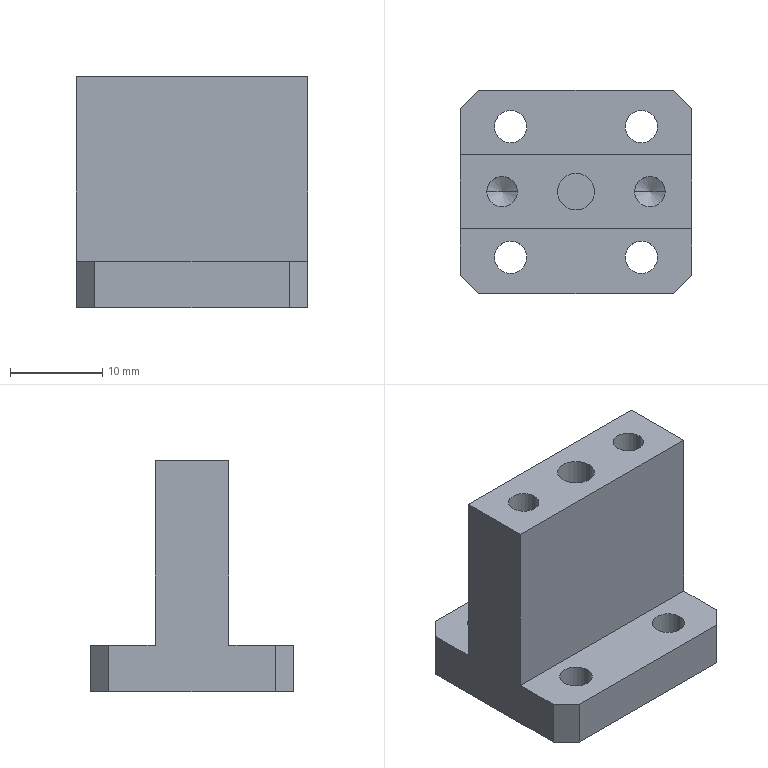Part | STEP file | 08-13 rotary support seat | 1 solid | 33 faces | box 25 x 22 x 25 mm | volume 6276 mm3 | plane 15 | cylinder 14 | cone 4 | commonest cylinder face diameters 3.5 x8 3.3 x4 4 x2
STEP:
#1=CARTESIAN_POINT('',(-9.65,0.,14.9));
#2=VERTEX_POINT('',#1);
#3=CARTESIAN_POINT('',(-6.35,0.,14.9));
#4=VERTEX_POINT('',#3);
#5=CARTESIAN_POINT('',(-8.,0.,14.9));
#6=DIRECTION('',(0.,0.,1.));
#7=DIRECTION('',(1.,0.,0.));
#8=AXIS2_PLACEMENT_3D('',#5,#6,#7);
#9=CIRCLE('',#8,1.65);
#10=EDGE_CURVE('',#2,#4,#9,.T.);
#11=ORIENTED_EDGE('',*,*,#10,.F.);
#12=CARTESIAN_POINT('',(-9.65,0.,25.));
#13=VERTEX_POINT('',#12);
#14=CARTESIAN_POINT('',(-9.65,0.,25.));
#15=DIRECTION('',(0.,0.,1.));
#16=VECTOR('',#15,1000.);
#17=LINE('',#14,#16);
#18=EDGE_CURVE('',#2,#13,#17,.T.);
#19=ORIENTED_EDGE('',*,*,#18,.T.);
#20=CARTESIAN_POINT('',(-6.35,0.,25.));
#21=VERTEX_POINT('',#20);
#22=CARTESIAN_POINT('',(-8.,0.,25.));
#23=DIRECTION('',(0.,0.,1.));
#24=DIRECTION('',(1.,0.,0.));
#25=AXIS2_PLACEMENT_3D('',#22,#23,#24);
#26=CIRCLE('',#25,1.65);
#27=EDGE_CURVE('',#13,#21,#26,.T.);
#28=ORIENTED_EDGE('',*,*,#27,.T.);
#29=CARTESIAN_POINT('',(-6.35,0.,25.));
#30=DIRECTION('',(0.,0.,1.));
#31=VECTOR('',#30,1000.);
#32=LINE('',#29,#31);
#33=EDGE_CURVE('',#4,#21,#32,.T.);
#34=ORIENTED_EDGE('',*,*,#33,.F.);
#35=EDGE_LOOP('',(#11,#19,#28,#34));
#36=FACE_OUTER_BOUND('',#35,.T.);
#37=CARTESIAN_POINT('',(-8.,0.,25.));
#38=DIRECTION('',(0.,0.,1.));
#39=DIRECTION('',(1.,0.,0.));
#40=AXIS2_PLACEMENT_3D('',#37,#38,#39);
#41=CYLINDRICAL_SURFACE('',#40,1.65);
#42=ADVANCED_FACE('',(#36),#41,.F.);
#43=CARTESIAN_POINT('',(-8.,0.,13.909));
#44=VERTEX_POINT('',#43);
#45=CARTESIAN_POINT('',(-6.35,0.,14.9));
#46=DIRECTION('',(0.8572,0.,0.515));
#47=VECTOR('',#46,1000.);
#48=LINE('',#45,#47);
#49=EDGE_CURVE('',#44,#4,#48,.T.);
#50=ORIENTED_EDGE('',*,*,#49,.F.);
#51=CARTESIAN_POINT('',(-9.65,0.,14.9));
#52=DIRECTION('',(-0.8572,0.,0.515));
#53=VECTOR('',#52,1000.);
#54=LINE('',#51,#53);
#55=EDGE_CURVE('',#44,#2,#54,.T.);
#56=ORIENTED_EDGE('',*,*,#55,.T.);
#57=ORIENTED_EDGE('',*,*,#10,.T.);
#58=EDGE_LOOP('',(#50,#56,#57));
#59=FACE_OUTER_BOUND('',#58,.T.);
#60=CARTESIAN_POINT('',(-8.,0.,14.9));
#61=DIRECTION('',(0.,0.,1.));
#62=DIRECTION('',(1.,0.,0.));
#63=AXIS2_PLACEMENT_3D('',#60,#61,#62);
#64=CONICAL_SURFACE('',#63,1.65,1.03);
#65=ADVANCED_FACE('',(#59),#64,.F.);
#66=CARTESIAN_POINT('',(6.35,0.,14.9));
#67=VERTEX_POINT('',#66);
#68=CARTESIAN_POINT('',(9.65,0.,14.9));
#69=VERTEX_POINT('',#68);
#70=CARTESIAN_POINT('',(8.,0.,14.9));
#71=DIRECTION('',(0.,0.,1.));
#72=DIRECTION('',(1.,0.,0.));
#73=AXIS2_PLACEMENT_3D('',#70,#71,#72);
#74=CIRCLE('',#73,1.65);
#75=EDGE_CURVE('',#67,#69,#74,.T.);
#76=ORIENTED_EDGE('',*,*,#75,.F.);
#77=CARTESIAN_POINT('',(6.35,0.,25.));
#78=VERTEX_POINT('',#77);
#79=CARTESIAN_POINT('',(6.35,0.,25.));
#80=DIRECTION('',(0.,0.,1.));
#81=VECTOR('',#80,1000.);
#82=LINE('',#79,#81);
#83=EDGE_CURVE('',#67,#78,#82,.T.);
#84=ORIENTED_EDGE('',*,*,#83,.T.);
#85=CARTESIAN_POINT('',(9.65,0.,25.));
#86=VERTEX_POINT('',#85);
#87=CARTESIAN_POINT('',(8.,0.,25.));
#88=DIRECTION('',(0.,0.,1.));
#89=DIRECTION('',(1.,0.,0.));
#90=AXIS2_PLACEMENT_3D('',#87,#88,#89);
#91=CIRCLE('',#90,1.65);
#92=EDGE_CURVE('',#78,#86,#91,.T.);
#93=ORIENTED_EDGE('',*,*,#92,.T.);
#94=CARTESIAN_POINT('',(9.65,0.,25.));
#95=DIRECTION('',(0.,0.,1.));
#96=VECTOR('',#95,1000.);
#97=LINE('',#94,#96);
#98=EDGE_CURVE('',#69,#86,#97,.T.);
#99=ORIENTED_EDGE('',*,*,#98,.F.);
#100=EDGE_LOOP('',(#76,#84,#93,#99));
#101=FACE_OUTER_BOUND('',#100,.T.);
#102=CARTESIAN_POINT('',(8.,0.,25.));
#103=DIRECTION('',(0.,0.,1.));
#104=DIRECTION('',(1.,0.,0.));
#105=AXIS2_PLACEMENT_3D('',#102,#103,#104);
#106=CYLINDRICAL_SURFACE('',#105,1.65);
#107=ADVANCED_FACE('',(#101),#106,.F.);
#108=CARTESIAN_POINT('',(8.,0.,13.909));
#109=VERTEX_POINT('',#108);
#110=CARTESIAN_POINT('',(9.65,0.,14.9));
#111=DIRECTION('',(0.8572,0.,0.515));
#112=VECTOR('',#111,1000.);
#113=LINE('',#110,#112);
#114=EDGE_CURVE('',#109,#69,#113,.T.);
#115=ORIENTED_EDGE('',*,*,#114,.F.);
#116=CARTESIAN_POINT('',(6.35,0.,14.9));
#117=DIRECTION('',(-0.8572,0.,0.515));
#118=VECTOR('',#117,1000.);
#119=LINE('',#116,#118);
#120=EDGE_CURVE('',#109,#67,#119,.T.);
#121=ORIENTED_EDGE('',*,*,#120,.T.);
#122=ORIENTED_EDGE('',*,*,#75,.T.);
#123=EDGE_LOOP('',(#115,#121,#122));
#124=FACE_OUTER_BOUND('',#123,.T.);
#125=CARTESIAN_POINT('',(8.,0.,14.9));
#126=DIRECTION('',(0.,0.,1.));
#127=DIRECTION('',(1.,0.,0.));
#128=AXIS2_PLACEMENT_3D('',#125,#126,#127);
#129=CONICAL_SURFACE('',#128,1.65,1.03);
#130=ADVANCED_FACE('',(#124),#129,.F.);
#131=CARTESIAN_POINT('',(-2.,0.,20.));
#132=VERTEX_POINT('',#131);
#133=CARTESIAN_POINT('',(2.,0.,20.));
#134=VERTEX_POINT('',#133);
#135=CARTESIAN_POINT('',(0.,0.,20.));
#136=DIRECTION('',(0.,0.,1.));
#137=DIRECTION('',(1.,0.,0.));
#138=AXIS2_PLACEMENT_3D('',#135,#136,#137);
#139=CIRCLE('',#138,2.);
#140=EDGE_CURVE('',#132,#134,#139,.T.);
#141=ORIENTED_EDGE('',*,*,#140,.F.);
#142=CARTESIAN_POINT('',(-2.,0.,25.));
#143=VERTEX_POINT('',#142);
#144=CARTESIAN_POINT('',(-2.,0.,20.));
#145=DIRECTION('',(0.,0.,1.));
#146=VECTOR('',#145,1000.);
#147=LINE('',#144,#146);
#148=EDGE_CURVE('',#132,#143,#147,.T.);
#149=ORIENTED_EDGE('',*,*,#148,.T.);
#150=CARTESIAN_POINT('',(2.,0.,25.));
#151=VERTEX_POINT('',#150);
#152=CARTESIAN_POINT('',(0.,0.,25.));
#153=DIRECTION('',(0.,0.,1.));
#154=DIRECTION('',(1.,0.,0.));
#155=AXIS2_PLACEMENT_3D('',#152,#153,#154);
#156=CIRCLE('',#155,2.);
#157=EDGE_CURVE('',#143,#151,#156,.T.);
#158=ORIENTED_EDGE('',*,*,#157,.T.);
#159=CARTESIAN_POINT('',(2.,0.,20.));
#160=DIRECTION('',(0.,0.,1.));
#161=VECTOR('',#160,1000.);
#162=LINE('',#159,#161);
#163=EDGE_CURVE('',#134,#151,#162,.T.);
#164=ORIENTED_EDGE('',*,*,#163,.F.);
#165=EDGE_LOOP('',(#141,#149,#158,#164));
#166=FACE_OUTER_BOUND('',#165,.T.);
#167=CARTESIAN_POINT('',(0.,0.,20.));
#168=DIRECTION('',(0.,0.,1.));
#169=DIRECTION('',(1.,0.,0.));
#170=AXIS2_PLACEMENT_3D('',#167,#168,#169);
#171=CYLINDRICAL_SURFACE('',#170,2.);
#172=ADVANCED_FACE('',(#166),#171,.F.);
#173=CARTESIAN_POINT('',(-8.821,-7.071,0.));
#174=VERTEX_POINT('',#173);
#175=CARTESIAN_POINT('',(-5.321,-7.071,0.));
#176=VERTEX_POINT('',#175);
#177=CARTESIAN_POINT('',(-7.071,-7.071,0.));
#178=DIRECTION('',(0.,0.,1.));
#179=DIRECTION('',(1.,0.,0.));
#180=AXIS2_PLACEMENT_3D('',#177,#178,#179);
#181=CIRCLE('',#180,1.75);
#182=EDGE_CURVE('',#174,#176,#181,.T.);
#183=ORIENTED_EDGE('',*,*,#182,.F.);
#184=CARTESIAN_POINT('',(-8.821,-7.071,5.));
#185=VERTEX_POINT('',#184);
#186=CARTESIAN_POINT('',(-8.821,-7.071,5.));
#187=DIRECTION('',(0.,0.,1.));
#188=VECTOR('',#187,1000.);
#189=LINE('',#186,#188);
#190=EDGE_CURVE('',#174,#185,#189,.T.);
#191=ORIENTED_EDGE('',*,*,#190,.T.);
#192=CARTESIAN_POINT('',(-5.321,-7.071,5.));
#193=VERTEX_POINT('',#192);
#194=CARTESIAN_POINT('',(-7.071,-7.071,5.));
#195=DIRECTION('',(0.,0.,1.));
#196=DIRECTION('',(1.,0.,0.));
#197=AXIS2_PLACEMENT_3D('',#194,#195,#196);
#198=CIRCLE('',#197,1.75);
#199=EDGE_CURVE('',#185,#193,#198,.T.);
#200=ORIENTED_EDGE('',*,*,#199,.T.);
#201=CARTESIAN_POINT('',(-5.321,-7.071,5.));
#202=DIRECTION('',(0.,0.,1.));
#203=VECTOR('',#202,1000.);
#204=LINE('',#201,#203);
#205=EDGE_CURVE('',#176,#193,#204,.T.);
#206=ORIENTED_EDGE('',*,*,#205,.F.);
#207=EDGE_LOOP('',(#183,#191,#200,#206));
#208=FACE_OUTER_BOUND('',#207,.T.);
#209=CARTESIAN_POINT('',(-7.071,-7.071,5.));
#210=DIRECTION('',(0.,0.,1.));
#211=DIRECTION('',(1.,0.,0.));
#212=AXIS2_PLACEMENT_3D('',#209,#210,#211);
#213=CYLINDRICAL_SURFACE('',#212,1.75);
#214=ADVANCED_FACE('',(#208),#213,.F.);
#215=CARTESIAN_POINT('',(5.321,-7.071,0.));
#216=VERTEX_POINT('',#215);
#217=CARTESIAN_POINT('',(8.821,-7.071,0.));
#218=VERTEX_POINT('',#217);
#219=CARTESIAN_POINT('',(7.071,-7.071,0.));
#220=DIRECTION('',(0.,0.,1.));
#221=DIRECTION('',(1.,0.,0.));
#222=AXIS2_PLACEMENT_3D('',#219,#220,#221);
#223=CIRCLE('',#222,1.75);
#224=EDGE_CURVE('',#216,#218,#223,.T.);
#225=ORIENTED_EDGE('',*,*,#224,.F.);
#226=CARTESIAN_POINT('',(5.321,-7.071,5.));
#227=VERTEX_POINT('',#226);
#228=CARTESIAN_POINT('',(5.321,-7.071,5.));
#229=DIRECTION('',(0.,0.,1.));
#230=VECTOR('',#229,1000.);
#231=LINE('',#228,#230);
#232=EDGE_CURVE('',#216,#227,#231,.T.);
#233=ORIENTED_EDGE('',*,*,#232,.T.);
#234=CARTESIAN_POINT('',(8.821,-7.071,5.));
#235=VERTEX_POINT('',#234);
#236=CARTESIAN_POINT('',(7.071,-7.071,5.));
#237=DIRECTION('',(0.,0.,1.));
#238=DIRECTION('',(1.,0.,0.));
#239=AXIS2_PLACEMENT_3D('',#236,#237,#238);
#240=CIRCLE('',#239,1.75);
#241=EDGE_CURVE('',#227,#235,#240,.T.);
#242=ORIENTED_EDGE('',*,*,#241,.T.);
#243=CARTESIAN_POINT('',(8.821,-7.071,5.));
#244=DIRECTION('',(0.,0.,1.));
#245=VECTOR('',#244,1000.);
#246=LINE('',#243,#245);
#247=EDGE_CURVE('',#218,#235,#246,.T.);
#248=ORIENTED_EDGE('',*,*,#247,.F.);
#249=EDGE_LOOP('',(#225,#233,#242,#248));
#250=FACE_OUTER_BOUND('',#249,.T.);
#251=CARTESIAN_POINT('',(7.071,-7.071,5.));
#252=DIRECTION('',(0.,0.,1.));
#253=DIRECTION('',(1.,0.,0.));
#254=AXIS2_PLACEMENT_3D('',#251,#252,#253);
#255=CYLINDRICAL_SURFACE('',#254,1.75);
#256=ADVANCED_FACE('',(#250),#255,.F.);
#257=CARTESIAN_POINT('',(5.321,7.071,0.));
#258=VERTEX_POINT('',#257);
#259=CARTESIAN_POINT('',(8.821,7.071,0.));
#260=VERTEX_POINT('',#259);
#261=CARTESIAN_POINT('',(7.071,7.071,0.));
#262=DIRECTION('',(0.,0.,1.));
#263=DIRECTION('',(1.,0.,0.));
#264=AXIS2_PLACEMENT_3D('',#261,#262,#263);
#265=CIRCLE('',#264,1.75);
#266=EDGE_CURVE('',#258,#260,#265,.T.);
#267=ORIENTED_EDGE('',*,*,#266,.F.);
#268=CARTESIAN_POINT('',(5.321,7.071,5.));
#269=VERTEX_POINT('',#268);
#270=CARTESIAN_POINT('',(5.321,7.071,5.));
#271=DIRECTION('',(0.,0.,1.));
#272=VECTOR('',#271,1000.);
#273=LINE('',#270,#272);
#274=EDGE_CURVE('',#258,#269,#273,.T.);
#275=ORIENTED_EDGE('',*,*,#274,.T.);
#276=CARTESIAN_POINT('',(8.821,7.071,5.));
#277=VERTEX_POINT('',#276);
#278=CARTESIAN_POINT('',(7.071,7.071,5.));
#279=DIRECTION('',(0.,0.,1.));
#280=DIRECTION('',(1.,0.,0.));
#281=AXIS2_PLACEMENT_3D('',#278,#279,#280);
#282=CIRCLE('',#281,1.75);
#283=EDGE_CURVE('',#269,#277,#282,.T.);
#284=ORIENTED_EDGE('',*,*,#283,.T.);
#285=CARTESIAN_POINT('',(8.821,7.071,5.));
#286=DIRECTION('',(0.,0.,1.));
#287=VECTOR('',#286,1000.);
#288=LINE('',#285,#287);
#289=EDGE_CURVE('',#260,#277,#288,.T.);
#290=ORIENTED_EDGE('',*,*,#289,.F.);
#291=EDGE_LOOP('',(#267,#275,#284,#290));
#292=FACE_OUTER_BOUND('',#291,.T.);
#293=CARTESIAN_POINT('',(7.071,7.071,5.));
#294=DIRECTION('',(0.,0.,1.));
#295=DIRECTION('',(1.,0.,0.));
#296=AXIS2_PLACEMENT_3D('',#293,#294,#295);
#297=CYLINDRICAL_SURFACE('',#296,1.75);
#298=ADVANCED_FACE('',(#292),#297,.F.);
#299=CARTESIAN_POINT('',(-8.821,7.071,0.));
#300=VERTEX_POINT('',#299);
#301=CARTESIAN_POINT('',(-5.321,7.071,0.));
#302=VERTEX_POINT('',#301);
#303=CARTESIAN_POINT('',(-7.071,7.071,0.));
#304=DIRECTION('',(0.,0.,1.));
#305=DIRECTION('',(1.,0.,0.));
#306=AXIS2_PLACEMENT_3D('',#303,#304,#305);
#307=CIRCLE('',#306,1.75);
#308=EDGE_CURVE('',#300,#302,#307,.T.);
#309=ORIENTED_EDGE('',*,*,#308,.F.);
#310=CARTESIAN_POINT('',(-8.821,7.071,5.));
#311=VERTEX_POINT('',#310);
#312=CARTESIAN_POINT('',(-8.821,7.071,5.));
#313=DIRECTION('',(0.,0.,1.));
#314=VECTOR('',#313,1000.);
#315=LINE('',#312,#314);
#316=EDGE_CURVE('',#300,#311,#315,.T.);
#317=ORIENTED_EDGE('',*,*,#316,.T.);
#318=CARTESIAN_POINT('',(-5.321,7.071,5.));
#319=VERTEX_POINT('',#318);
#320=CARTESIAN_POINT('',(-7.071,7.071,5.));
#321=DIRECTION('',(0.,0.,1.));
#322=DIRECTION('',(1.,0.,0.));
#323=AXIS2_PLACEMENT_3D('',#320,#321,#322);
#324=CIRCLE('',#323,1.75);
#325=EDGE_CURVE('',#311,#319,#324,.T.);
#326=ORIENTED_EDGE('',*,*,#325,.T.);
#327=CARTESIAN_POINT('',(-5.321,7.071,5.));
#328=DIRECTION('',(0.,0.,1.));
#329=VECTOR('',#328,1000.);
#330=LINE('',#327,#329);
#331=EDGE_CURVE('',#302,#319,#330,.T.);
#332=ORIENTED_EDGE('',*,*,#331,.F.);
#333=EDGE_LOOP('',(#309,#317,#326,#332));
#334=FACE_OUTER_BOUND('',#333,.T.);
#335=CARTESIAN_POINT('',(-7.071,7.071,5.));
#336=DIRECTION('',(0.,0.,1.));
#337=DIRECTION('',(1.,0.,0.));
#338=AXIS2_PLACEMENT_3D('',#335,#336,#337);
#339=CYLINDRICAL_SURFACE('',#338,1.75);
#340=ADVANCED_FACE('',(#334),#339,.F.);
#341=CARTESIAN_POINT('',(-12.5,-4.,5.));
#342=VERTEX_POINT('',#341);
#343=CARTESIAN_POINT('',(-12.5,-9.,5.));
#344=VERTEX_POINT('',#343);
#345=CARTESIAN_POINT('',(-12.5,11.,5.));
#346=DIRECTION('',(0.,-1.,0.));
#347=VECTOR('',#346,1000.);
#348=LINE('',#345,#347);
#349=EDGE_CURVE('',#342,#344,#348,.T.);
#350=ORIENTED_EDGE('',*,*,#349,.T.);
#351=CARTESIAN_POINT('',(-10.5,-11.,5.));
#352=VERTEX_POINT('',#351);
#353=CARTESIAN_POINT('',(1.,-22.5,5.));
#354=DIRECTION('',(0.7071,-0.7071,0.));
#355=VECTOR('',#354,1000.);
#356=LINE('',#353,#355);
#357=EDGE_CURVE('',#344,#352,#356,.T.);
#358=ORIENTED_EDGE('',*,*,#357,.T.);
#359=CARTESIAN_POINT('',(10.5,-11.,5.));
#360=VERTEX_POINT('',#359);
#361=CARTESIAN_POINT('',(-12.5,-11.,5.));
#362=DIRECTION('',(1.,0.,0.));
#363=VECTOR('',#362,1000.);
#364=LINE('',#361,#363);
#365=EDGE_CURVE('',#352,#360,#364,.T.);
#366=ORIENTED_EDGE('',*,*,#365,.T.);
#367=CARTESIAN_POINT('',(12.5,-9.,5.));
#368=VERTEX_POINT('',#367);
#369=CARTESIAN_POINT('',(11.5,-10.,5.));
#370=DIRECTION('',(0.7071,0.7071,0.));
#371=VECTOR('',#370,1000.);
#372=LINE('',#369,#371);
#373=EDGE_CURVE('',#360,#368,#372,.T.);
#374=ORIENTED_EDGE('',*,*,#373,.T.);
#375=CARTESIAN_POINT('',(12.5,-4.,5.));
#376=VERTEX_POINT('',#375);
#377=CARTESIAN_POINT('',(12.5,11.,5.));
#378=DIRECTION('',(0.,1.,0.));
#379=VECTOR('',#378,1000.);
#380=LINE('',#377,#379);
#381=EDGE_CURVE('',#368,#376,#380,.T.);
#382=ORIENTED_EDGE('',*,*,#381,.T.);
#383=CARTESIAN_POINT('',(-12.5,-4.,5.));
#384=DIRECTION('',(1.,0.,0.));
#385=VECTOR('',#384,1000.);
#386=LINE('',#383,#385);
#387=EDGE_CURVE('',#342,#376,#386,.T.);
#388=ORIENTED_EDGE('',*,*,#387,.F.);
#389=EDGE_LOOP('',(#350,#358,#366,#374,#382,#388));
#390=FACE_OUTER_BOUND('',#389,.T.);
#391=CARTESIAN_POINT('',(7.071,-7.071,5.));
#392=DIRECTION('',(0.,0.,1.));
#393=DIRECTION('',(1.,0.,0.));
#394=AXIS2_PLACEMENT_3D('',#391,#392,#393);
#395=CIRCLE('',#394,1.75);
#396=EDGE_CURVE('',#235,#227,#395,.T.);
#397=ORIENTED_EDGE('',*,*,#396,.F.);
#398=ORIENTED_EDGE('',*,*,#241,.F.);
#399=EDGE_LOOP('',(#397,#398));
#400=FACE_BOUND('',#399,.T.);
#401=CARTESIAN_POINT('',(-7.071,-7.071,5.));
#402=DIRECTION('',(0.,0.,1.));
#403=DIRECTION('',(1.,0.,0.));
#404=AXIS2_PLACEMENT_3D('',#401,#402,#403);
#405=CIRCLE('',#404,1.75);
#406=EDGE_CURVE('',#193,#185,#405,.T.);
#407=ORIENTED_EDGE('',*,*,#406,.F.);
#408=ORIENTED_EDGE('',*,*,#199,.F.);
#409=EDGE_LOOP('',(#407,#408));
#410=FACE_BOUND('',#409,.T.);
#411=CARTESIAN_POINT('',(12.5,-11.,5.));
#412=DIRECTION('',(0.,0.,1.));
#413=DIRECTION('',(1.,0.,0.));
#414=AXIS2_PLACEMENT_3D('',#411,#412,#413);
#415=PLANE('',#414);
#416=ADVANCED_FACE('',(#390,#400,#410),#415,.T.);
#417=ORIENTED_EDGE('',*,*,#381,.F.);
#418=CARTESIAN_POINT('',(12.5,-9.,0.));
#419=VERTEX_POINT('',#418);
#420=CARTESIAN_POINT('',(12.5,-9.,5.));
#421=DIRECTION('',(0.,0.,-1.));
#422=VECTOR('',#421,1000.);
#423=LINE('',#420,#422);
#424=EDGE_CURVE('',#368,#419,#423,.T.);
#425=ORIENTED_EDGE('',*,*,#424,.T.);
#426=CARTESIAN_POINT('',(12.5,9.,0.));
#427=VERTEX_POINT('',#426);
#428=CARTESIAN_POINT('',(12.5,11.,0.));
#429=DIRECTION('',(0.,1.,0.));
#430=VECTOR('',#429,1000.);
#431=LINE('',#428,#430);
#432=EDGE_CURVE('',#419,#427,#431,.T.);
#433=ORIENTED_EDGE('',*,*,#432,.T.);
#434=CARTESIAN_POINT('',(12.5,9.,5.));
#435=VERTEX_POINT('',#434);
#436=CARTESIAN_POINT('',(12.5,9.,5.));
#437=DIRECTION('',(0.,0.,1.));
#438=VECTOR('',#437,1000.);
#439=LINE('',#436,#438);
#440=EDGE_CURVE('',#427,#435,#439,.T.);
#441=ORIENTED_EDGE('',*,*,#440,.T.);
#442=CARTESIAN_POINT('',(12.5,4.,5.));
#443=VERTEX_POINT('',#442);
#444=CARTESIAN_POINT('',(12.5,11.,5.));
#445=DIRECTION('',(0.,1.,0.));
#446=VECTOR('',#445,1000.);
#447=LINE('',#444,#446);
#448=EDGE_CURVE('',#443,#435,#447,.T.);
#449=ORIENTED_EDGE('',*,*,#448,.F.);
#450=CARTESIAN_POINT('',(12.5,4.,25.));
#451=VERTEX_POINT('',#450);
#452=CARTESIAN_POINT('',(12.5,4.,25.));
#453=DIRECTION('',(0.,0.,-1.));
#454=VECTOR('',#453,1000.);
#455=LINE('',#452,#454);
#456=EDGE_CURVE('',#451,#443,#455,.T.);
#457=ORIENTED_EDGE('',*,*,#456,.F.);
#458=CARTESIAN_POINT('',(12.5,-4.,25.));
#459=VERTEX_POINT('',#458);
#460=CARTESIAN_POINT('',(12.5,4.,25.));
#461=DIRECTION('',(0.,1.,0.));
#462=VECTOR('',#461,1000.);
#463=LINE('',#460,#462);
#464=EDGE_CURVE('',#459,#451,#463,.T.);
#465=ORIENTED_EDGE('',*,*,#464,.F.);
#466=CARTESIAN_POINT('',(12.5,-4.,25.));
#467=DIRECTION('',(0.,0.,-1.));
#468=VECTOR('',#467,1000.);
#469=LINE('',#466,#468);
#470=EDGE_CURVE('',#459,#376,#469,.T.);
#471=ORIENTED_EDGE('',*,*,#470,.T.);
#472=EDGE_LOOP('',(#417,#425,#433,#441,#449,#457,#465,#471));
#473=FACE_OUTER_BOUND('',#472,.T.);
#474=CARTESIAN_POINT('',(12.5,11.,5.));
#475=DIRECTION('',(-1.,0.,0.));
#476=DIRECTION('',(0.,-1.,0.));
#477=AXIS2_PLACEMENT_3D('',#474,#475,#476);
#478=PLANE('',#477);
#479=ADVANCED_FACE('',(#473),#478,.F.);
#480=CARTESIAN_POINT('',(10.5,11.,5.));
#481=VERTEX_POINT('',#480);
#482=CARTESIAN_POINT('',(-10.5,11.,5.));
#483=VERTEX_POINT('',#482);
#484=CARTESIAN_POINT('',(-12.5,11.,5.));
#485=DIRECTION('',(-1.,0.,0.));
#486=VECTOR('',#485,1000.);
#487=LINE('',#484,#486);
#488=EDGE_CURVE('',#481,#483,#487,.T.);
#489=ORIENTED_EDGE('',*,*,#488,.F.);
#490=CARTESIAN_POINT('',(10.5,11.,0.));
#491=VERTEX_POINT('',#490);
#492=CARTESIAN_POINT('',(10.5,11.,5.));
#493=DIRECTION('',(0.,0.,-1.));
#494=VECTOR('',#493,1000.);
#495=LINE('',#492,#494);
#496=EDGE_CURVE('',#481,#491,#495,.T.);
#497=ORIENTED_EDGE('',*,*,#496,.T.);
#498=CARTESIAN_POINT('',(-10.5,11.,0.));
#499=VERTEX_POINT('',#498);
#500=CARTESIAN_POINT('',(-12.5,11.,0.));
#501=DIRECTION('',(-1.,0.,0.));
#502=VECTOR('',#501,1000.);
#503=LINE('',#500,#502);
#504=EDGE_CURVE('',#491,#499,#503,.T.);
#505=ORIENTED_EDGE('',*,*,#504,.T.);
#506=CARTESIAN_POINT('',(-10.5,11.,5.));
#507=DIRECTION('',(0.,0.,1.));
#508=VECTOR('',#507,1000.);
#509=LINE('',#506,#508);
#510=EDGE_CURVE('',#499,#483,#509,.T.);
#511=ORIENTED_EDGE('',*,*,#510,.T.);
#512=EDGE_LOOP('',(#489,#497,#505,#511));
#513=FACE_OUTER_BOUND('',#512,.T.);
#514=CARTESIAN_POINT('',(-12.5,11.,5.));
#515=DIRECTION('',(0.,-1.,0.));
#516=DIRECTION('',(0.,0.,-1.));
#517=AXIS2_PLACEMENT_3D('',#514,#515,#516);
#518=PLANE('',#517);
#519=ADVANCED_FACE('',(#513),#518,.F.);
#520=CARTESIAN_POINT('',(-12.5,9.,0.));
#521=VERTEX_POINT('',#520);
#522=CARTESIAN_POINT('',(-12.5,-9.,0.));
#523=VERTEX_POINT('',#522);
#524=CARTESIAN_POINT('',(-12.5,11.,0.));
#525=DIRECTION('',(0.,-1.,0.));
#526=VECTOR('',#525,1000.);
#527=LINE('',#524,#526);
#528=EDGE_CURVE('',#521,#523,#527,.T.);
#529=ORIENTED_EDGE('',*,*,#528,.T.);
#530=CARTESIAN_POINT('',(-12.5,-9.,5.));
#531=DIRECTION('',(0.,0.,1.));
#532=VECTOR('',#531,1000.);
#533=LINE('',#530,#532);
#534=EDGE_CURVE('',#523,#344,#533,.T.);
#535=ORIENTED_EDGE('',*,*,#534,.T.);
#536=ORIENTED_EDGE('',*,*,#349,.F.);
#537=CARTESIAN_POINT('',(-12.5,-4.,25.));
#538=VERTEX_POINT('',#537);
#539=CARTESIAN_POINT('',(-12.5,-4.,25.));
#540=DIRECTION('',(0.,0.,-1.));
#541=VECTOR('',#540,1000.);
#542=LINE('',#539,#541);
#543=EDGE_CURVE('',#538,#342,#542,.T.);
#544=ORIENTED_EDGE('',*,*,#543,.F.);
#545=CARTESIAN_POINT('',(-12.5,4.,25.));
#546=VERTEX_POINT('',#545);
#547=CARTESIAN_POINT('',(-12.5,4.,25.));
#548=DIRECTION('',(0.,-1.,0.));
#549=VECTOR('',#548,1000.);
#550=LINE('',#547,#549);
#551=EDGE_CURVE('',#546,#538,#550,.T.);
#552=ORIENTED_EDGE('',*,*,#551,.F.);
#553=CARTESIAN_POINT('',(-12.5,4.,5.));
#554=VERTEX_POINT('',#553);
#555=CARTESIAN_POINT('',(-12.5,4.,25.));
#556=DIRECTION('',(0.,0.,-1.));
#557=VECTOR('',#556,1000.);
#558=LINE('',#555,#557);
#559=EDGE_CURVE('',#546,#554,#558,.T.);
#560=ORIENTED_EDGE('',*,*,#559,.T.);
#561=CARTESIAN_POINT('',(-12.5,9.,5.));
#562=VERTEX_POINT('',#561);
#563=CARTESIAN_POINT('',(-12.5,11.,5.));
#564=DIRECTION('',(0.,-1.,0.));
#565=VECTOR('',#564,1000.);
#566=LINE('',#563,#565);
#567=EDGE_CURVE('',#562,#554,#566,.T.);
#568=ORIENTED_EDGE('',*,*,#567,.F.);
#569=CARTESIAN_POINT('',(-12.5,9.,5.));
#570=DIRECTION('',(0.,0.,-1.));
#571=VECTOR('',#570,1000.);
#572=LINE('',#569,#571);
#573=EDGE_CURVE('',#562,#521,#572,.T.);
#574=ORIENTED_EDGE('',*,*,#573,.T.);
#575=EDGE_LOOP('',(#529,#535,#536,#544,#552,#560,#568,#574));
#576=FACE_OUTER_BOUND('',#575,.T.);
#577=CARTESIAN_POINT('',(-12.5,11.,5.));
#578=DIRECTION('',(1.,0.,0.));
#579=DIRECTION('',(0.,1.,0.));
#580=AXIS2_PLACEMENT_3D('',#577,#578,#579);
#581=PLANE('',#580);
#582=ADVANCED_FACE('',(#576),#581,.F.);
#583=ORIENTED_EDGE('',*,*,#365,.F.);
#584=CARTESIAN_POINT('',(-10.5,-11.,0.));
#585=VERTEX_POINT('',#584);
#586=CARTESIAN_POINT('',(-10.5,-11.,5.));
#587=DIRECTION('',(0.,0.,-1.));
#588=VECTOR('',#587,1000.);
#589=LINE('',#586,#588);
#590=EDGE_CURVE('',#352,#585,#589,.T.);
#591=ORIENTED_EDGE('',*,*,#590,.T.);
#592=CARTESIAN_POINT('',(10.5,-11.,0.));
#593=VERTEX_POINT('',#592);
#594=CARTESIAN_POINT('',(-12.5,-11.,0.));
#595=DIRECTION('',(1.,0.,0.));
#596=VECTOR('',#595,1000.);
#597=LINE('',#594,#596);
#598=EDGE_CURVE('',#585,#593,#597,.T.);
#599=ORIENTED_EDGE('',*,*,#598,.T.);
#600=CARTESIAN_POINT('',(10.5,-11.,5.));
#601=DIRECTION('',(0.,0.,1.));
#602=VECTOR('',#601,1000.);
#603=LINE('',#600,#602);
#604=EDGE_CURVE('',#593,#360,#603,.T.);
#605=ORIENTED_EDGE('',*,*,#604,.T.);
#606=EDGE_LOOP('',(#583,#591,#599,#605));
#607=FACE_OUTER_BOUND('',#606,.T.);
#608=CARTESIAN_POINT('',(-12.5,-11.,5.));
#609=DIRECTION('',(0.,1.,0.));
#610=DIRECTION('',(0.,0.,1.));
#611=AXIS2_PLACEMENT_3D('',#608,#609,#610);
#612=PLANE('',#611);
#613=ADVANCED_FACE('',(#607),#612,.F.);
#614=ORIENTED_EDGE('',*,*,#448,.T.);
#615=CARTESIAN_POINT('',(22.5,-1.,5.));
#616=DIRECTION('',(-0.7071,0.7071,0.));
#617=VECTOR('',#616,1000.);
#618=LINE('',#615,#617);
#619=EDGE_CURVE('',#435,#481,#618,.T.);
#620=ORIENTED_EDGE('',*,*,#619,.T.);
#621=ORIENTED_EDGE('',*,*,#488,.T.);
#622=CARTESIAN_POINT('',(-10.,11.5,5.));
#623=DIRECTION('',(-0.7071,-0.7071,0.));
#624=VECTOR('',#623,1000.);
#625=LINE('',#622,#624);
#626=EDGE_CURVE('',#483,#562,#625,.T.);
#627=ORIENTED_EDGE('',*,*,#626,.T.);
#628=ORIENTED_EDGE('',*,*,#567,.T.);
#629=CARTESIAN_POINT('',(-12.5,4.,5.));
#630=DIRECTION('',(-1.,0.,0.));
#631=VECTOR('',#630,1000.);
#632=LINE('',#629,#631);
#633=EDGE_CURVE('',#443,#554,#632,.T.);
#634=ORIENTED_EDGE('',*,*,#633,.F.);
#635=EDGE_LOOP('',(#614,#620,#621,#627,#628,#634));
#636=FACE_OUTER_BOUND('',#635,.T.);
#637=CARTESIAN_POINT('',(7.071,7.071,5.));
#638=DIRECTION('',(0.,0.,1.));
#639=DIRECTION('',(1.,0.,0.));
#640=AXIS2_PLACEMENT_3D('',#637,#638,#639);
#641=CIRCLE('',#640,1.75);
#642=EDGE_CURVE('',#277,#269,#641,.T.);
#643=ORIENTED_EDGE('',*,*,#642,.F.);
#644=ORIENTED_EDGE('',*,*,#283,.F.);
#645=EDGE_LOOP('',(#643,#644));
#646=FACE_BOUND('',#645,.T.);
#647=CARTESIAN_POINT('',(-7.071,7.071,5.));
#648=DIRECTION('',(0.,0.,1.));
#649=DIRECTION('',(1.,0.,0.));
#650=AXIS2_PLACEMENT_3D('',#647,#648,#649);
#651=CIRCLE('',#650,1.75);
#652=EDGE_CURVE('',#319,#311,#651,.T.);
#653=ORIENTED_EDGE('',*,*,#652,.F.);
#654=ORIENTED_EDGE('',*,*,#325,.F.);
#655=EDGE_LOOP('',(#653,#654));
#656=FACE_BOUND('',#655,.T.);
#657=CARTESIAN_POINT('',(12.5,-11.,5.));
#658=DIRECTION('',(0.,0.,1.));
#659=DIRECTION('',(1.,0.,0.));
#660=AXIS2_PLACEMENT_3D('',#657,#658,#659);
#661=PLANE('',#660);
#662=ADVANCED_FACE('',(#636,#646,#656),#661,.T.);
#663=CARTESIAN_POINT('',(-7.071,-7.071,0.));
#664=DIRECTION('',(0.,0.,1.));
#665=DIRECTION('',(1.,0.,0.));
#666=AXIS2_PLACEMENT_3D('',#663,#664,#665);
#667=CIRCLE('',#666,1.75);
#668=EDGE_CURVE('',#176,#174,#667,.T.);
#669=ORIENTED_EDGE('',*,*,#668,.T.);
#670=ORIENTED_EDGE('',*,*,#182,.T.);
#671=EDGE_LOOP('',(#669,#670));
#672=FACE_BOUND('',#671,.T.);
#673=CARTESIAN_POINT('',(7.071,-7.071,0.));
#674=DIRECTION('',(0.,0.,1.));
#675=DIRECTION('',(1.,0.,0.));
#676=AXIS2_PLACEMENT_3D('',#673,#674,#675);
#677=CIRCLE('',#676,1.75);
#678=EDGE_CURVE('',#218,#216,#677,.T.);
#679=ORIENTED_EDGE('',*,*,#678,.T.);
#680=ORIENTED_EDGE('',*,*,#224,.T.);
#681=EDGE_LOOP('',(#679,#680));
#682=FACE_BOUND('',#681,.T.);
#683=CARTESIAN_POINT('',(7.071,7.071,0.));
#684=DIRECTION('',(0.,0.,1.));
#685=DIRECTION('',(1.,0.,0.));
#686=AXIS2_PLACEMENT_3D('',#683,#684,#685);
#687=CIRCLE('',#686,1.75);
#688=EDGE_CURVE('',#260,#258,#687,.T.);
#689=ORIENTED_EDGE('',*,*,#688,.T.);
#690=ORIENTED_EDGE('',*,*,#266,.T.);
#691=EDGE_LOOP('',(#689,#690));
#692=FACE_BOUND('',#691,.T.);
#693=CARTESIAN_POINT('',(-7.071,7.071,0.));
#694=DIRECTION('',(0.,0.,1.));
#695=DIRECTION('',(1.,0.,0.));
#696=AXIS2_PLACEMENT_3D('',#693,#694,#695);
#697=CIRCLE('',#696,1.75);
#698=EDGE_CURVE('',#302,#300,#697,.T.);
#699=ORIENTED_EDGE('',*,*,#698,.T.);
#700=ORIENTED_EDGE('',*,*,#308,.T.);
#701=EDGE_LOOP('',(#699,#700));
#702=FACE_BOUND('',#701,.T.);
#703=ORIENTED_EDGE('',*,*,#598,.F.);
#704=CARTESIAN_POINT('',(-10.5,-11.,0.));
#705=DIRECTION('',(-0.7071,0.7071,0.));
#706=VECTOR('',#705,1000.);
#707=LINE('',#704,#706);
#708=EDGE_CURVE('',#585,#523,#707,.T.);
#709=ORIENTED_EDGE('',*,*,#708,.T.);
#710=ORIENTED_EDGE('',*,*,#528,.F.);
#711=CARTESIAN_POINT('',(-12.5,9.,0.));
#712=DIRECTION('',(0.7071,0.7071,0.));
#713=VECTOR('',#712,1000.);
#714=LINE('',#711,#713);
#715=EDGE_CURVE('',#521,#499,#714,.T.);
#716=ORIENTED_EDGE('',*,*,#715,.T.);
#717=ORIENTED_EDGE('',*,*,#504,.F.);
#718=CARTESIAN_POINT('',(10.5,11.,0.));
#719=DIRECTION('',(0.7071,-0.7071,0.));
#720=VECTOR('',#719,1000.);
#721=LINE('',#718,#720);
#722=EDGE_CURVE('',#491,#427,#721,.T.);
#723=ORIENTED_EDGE('',*,*,#722,.T.);
#724=ORIENTED_EDGE('',*,*,#432,.F.);
#725=CARTESIAN_POINT('',(12.5,-9.,0.));
#726=DIRECTION('',(-0.7071,-0.7071,0.));
#727=VECTOR('',#726,1000.);
#728=LINE('',#725,#727);
#729=EDGE_CURVE('',#419,#593,#728,.T.);
#730=ORIENTED_EDGE('',*,*,#729,.T.);
#731=EDGE_LOOP('',(#703,#709,#710,#716,#717,#723,#724,#730));
#732=FACE_OUTER_BOUND('',#731,.T.);
#733=CARTESIAN_POINT('',(12.5,-11.,0.));
#734=DIRECTION('',(0.,0.,1.));
#735=DIRECTION('',(1.,0.,0.));
#736=AXIS2_PLACEMENT_3D('',#733,#734,#735);
#737=PLANE('',#736);
#738=ADVANCED_FACE('',(#672,#682,#692,#702,#732),#737,.F.);
#739=ORIENTED_EDGE('',*,*,#316,.F.);
#740=ORIENTED_EDGE('',*,*,#698,.F.);
#741=ORIENTED_EDGE('',*,*,#331,.T.);
#742=ORIENTED_EDGE('',*,*,#652,.T.);
#743=EDGE_LOOP('',(#739,#740,#741,#742));
#744=FACE_OUTER_BOUND('',#743,.T.);
#745=CARTESIAN_POINT('',(-7.071,7.071,5.));
#746=DIRECTION('',(0.,0.,1.));
#747=DIRECTION('',(1.,0.,0.));
#748=AXIS2_PLACEMENT_3D('',#745,#746,#747);
#749=CYLINDRICAL_SURFACE('',#748,1.75);
#750=ADVANCED_FACE('',(#744),#749,.F.);
#751=ORIENTED_EDGE('',*,*,#274,.F.);
#752=ORIENTED_EDGE('',*,*,#688,.F.);
#753=ORIENTED_EDGE('',*,*,#289,.T.);
#754=ORIENTED_EDGE('',*,*,#642,.T.);
#755=EDGE_LOOP('',(#751,#752,#753,#754));
#756=FACE_OUTER_BOUND('',#755,.T.);
#757=CARTESIAN_POINT('',(7.071,7.071,5.));
#758=DIRECTION('',(0.,0.,1.));
#759=DIRECTION('',(1.,0.,0.));
#760=AXIS2_PLACEMENT_3D('',#757,#758,#759);
#761=CYLINDRICAL_SURFACE('',#760,1.75);
#762=ADVANCED_FACE('',(#756),#761,.F.);
#763=ORIENTED_EDGE('',*,*,#232,.F.);
#764=ORIENTED_EDGE('',*,*,#678,.F.);
#765=ORIENTED_EDGE('',*,*,#247,.T.);
#766=ORIENTED_EDGE('',*,*,#396,.T.);
#767=EDGE_LOOP('',(#763,#764,#765,#766));
#768=FACE_OUTER_BOUND('',#767,.T.);
#769=CARTESIAN_POINT('',(7.071,-7.071,5.));
#770=DIRECTION('',(0.,0.,1.));
#771=DIRECTION('',(1.,0.,0.));
#772=AXIS2_PLACEMENT_3D('',#769,#770,#771);
#773=CYLINDRICAL_SURFACE('',#772,1.75);
#774=ADVANCED_FACE('',(#768),#773,.F.);
#775=ORIENTED_EDGE('',*,*,#190,.F.);
#776=ORIENTED_EDGE('',*,*,#668,.F.);
#777=ORIENTED_EDGE('',*,*,#205,.T.);
#778=ORIENTED_EDGE('',*,*,#406,.T.);
#779=EDGE_LOOP('',(#775,#776,#777,#778));
#780=FACE_OUTER_BOUND('',#779,.T.);
#781=CARTESIAN_POINT('',(-7.071,-7.071,5.));
#782=DIRECTION('',(0.,0.,1.));
#783=DIRECTION('',(1.,0.,0.));
#784=AXIS2_PLACEMENT_3D('',#781,#782,#783);
#785=CYLINDRICAL_SURFACE('',#784,1.75);
#786=ADVANCED_FACE('',(#780),#785,.F.);
#787=ORIENTED_EDGE('',*,*,#633,.T.);
#788=ORIENTED_EDGE('',*,*,#559,.F.);
#789=CARTESIAN_POINT('',(-12.5,4.,25.));
#790=DIRECTION('',(-1.,0.,0.));
#791=VECTOR('',#790,1000.);
#792=LINE('',#789,#791);
#793=EDGE_CURVE('',#451,#546,#792,.T.);
#794=ORIENTED_EDGE('',*,*,#793,.F.);
#795=ORIENTED_EDGE('',*,*,#456,.T.);
#796=EDGE_LOOP('',(#787,#788,#794,#795));
#797=FACE_OUTER_BOUND('',#796,.T.);
#798=CARTESIAN_POINT('',(-12.5,4.,25.));
#799=DIRECTION('',(0.,-1.,0.));
#800=DIRECTION('',(0.,0.,-1.));
#801=AXIS2_PLACEMENT_3D('',#798,#799,#800);
#802=PLANE('',#801);
#803=ADVANCED_FACE('',(#797),#802,.F.);
#804=ORIENTED_EDGE('',*,*,#387,.T.);
#805=ORIENTED_EDGE('',*,*,#470,.F.);
#806=CARTESIAN_POINT('',(-12.5,-4.,25.));
#807=DIRECTION('',(1.,0.,0.));
#808=VECTOR('',#807,1000.);
#809=LINE('',#806,#808);
#810=EDGE_CURVE('',#538,#459,#809,.T.);
#811=ORIENTED_EDGE('',*,*,#810,.F.);
#812=ORIENTED_EDGE('',*,*,#543,.T.);
#813=EDGE_LOOP('',(#804,#805,#811,#812));
#814=FACE_OUTER_BOUND('',#813,.T.);
#815=CARTESIAN_POINT('',(-12.5,-4.,25.));
#816=DIRECTION('',(0.,1.,0.));
#817=DIRECTION('',(0.,0.,1.));
#818=AXIS2_PLACEMENT_3D('',#815,#816,#817);
#819=PLANE('',#818);
#820=ADVANCED_FACE('',(#814),#819,.F.);
#821=CARTESIAN_POINT('',(-8.,0.,25.));
#822=DIRECTION('',(0.,0.,1.));
#823=DIRECTION('',(1.,0.,0.));
#824=AXIS2_PLACEMENT_3D('',#821,#822,#823);
#825=CIRCLE('',#824,1.65);
#826=EDGE_CURVE('',#21,#13,#825,.T.);
#827=ORIENTED_EDGE('',*,*,#826,.F.);
#828=ORIENTED_EDGE('',*,*,#27,.F.);
#829=EDGE_LOOP('',(#827,#828));
#830=FACE_BOUND('',#829,.T.);
#831=CARTESIAN_POINT('',(8.,0.,25.));
#832=DIRECTION('',(0.,0.,1.));
#833=DIRECTION('',(1.,0.,0.));
#834=AXIS2_PLACEMENT_3D('',#831,#832,#833);
#835=CIRCLE('',#834,1.65);
#836=EDGE_CURVE('',#86,#78,#835,.T.);
#837=ORIENTED_EDGE('',*,*,#836,.F.);
#838=ORIENTED_EDGE('',*,*,#92,.F.);
#839=EDGE_LOOP('',(#837,#838));
#840=FACE_BOUND('',#839,.T.);
#841=CARTESIAN_POINT('',(0.,0.,25.));
#842=DIRECTION('',(0.,0.,1.));
#843=DIRECTION('',(1.,0.,0.));
#844=AXIS2_PLACEMENT_3D('',#841,#842,#843);
#845=CIRCLE('',#844,2.);
#846=EDGE_CURVE('',#151,#143,#845,.T.);
#847=ORIENTED_EDGE('',*,*,#846,.F.);
#848=ORIENTED_EDGE('',*,*,#157,.F.);
#849=EDGE_LOOP('',(#847,#848));
#850=FACE_BOUND('',#849,.T.);
#851=ORIENTED_EDGE('',*,*,#464,.T.);
#852=ORIENTED_EDGE('',*,*,#793,.T.);
#853=ORIENTED_EDGE('',*,*,#551,.T.);
#854=ORIENTED_EDGE('',*,*,#810,.T.);
#855=EDGE_LOOP('',(#851,#852,#853,#854));
#856=FACE_OUTER_BOUND('',#855,.T.);
#857=CARTESIAN_POINT('',(12.5,-4.,25.));
#858=DIRECTION('',(0.,0.,1.));
#859=DIRECTION('',(1.,0.,0.));
#860=AXIS2_PLACEMENT_3D('',#857,#858,#859);
#861=PLANE('',#860);
#862=ADVANCED_FACE('',(#830,#840,#850,#856),#861,.T.);
#863=ORIENTED_EDGE('',*,*,#357,.F.);
#864=ORIENTED_EDGE('',*,*,#534,.F.);
#865=ORIENTED_EDGE('',*,*,#708,.F.);
#866=ORIENTED_EDGE('',*,*,#590,.F.);
#867=EDGE_LOOP('',(#863,#864,#865,#866));
#868=FACE_OUTER_BOUND('',#867,.T.);
#869=CARTESIAN_POINT('',(-10.5,-11.,5.));
#870=DIRECTION('',(0.7071,0.7071,0.));
#871=DIRECTION('',(-0.7071,0.7071,0.));
#872=AXIS2_PLACEMENT_3D('',#869,#870,#871);
#873=PLANE('',#872);
#874=ADVANCED_FACE('',(#868),#873,.F.);
#875=ORIENTED_EDGE('',*,*,#373,.F.);
#876=ORIENTED_EDGE('',*,*,#604,.F.);
#877=ORIENTED_EDGE('',*,*,#729,.F.);
#878=ORIENTED_EDGE('',*,*,#424,.F.);
#879=EDGE_LOOP('',(#875,#876,#877,#878));
#880=FACE_OUTER_BOUND('',#879,.T.);
#881=CARTESIAN_POINT('',(12.5,-9.,5.));
#882=DIRECTION('',(-0.7071,0.7071,0.));
#883=DIRECTION('',(-0.7071,-0.7071,0.));
#884=AXIS2_PLACEMENT_3D('',#881,#882,#883);
#885=PLANE('',#884);
#886=ADVANCED_FACE('',(#880),#885,.F.);
#887=ORIENTED_EDGE('',*,*,#619,.F.);
#888=ORIENTED_EDGE('',*,*,#440,.F.);
#889=ORIENTED_EDGE('',*,*,#722,.F.);
#890=ORIENTED_EDGE('',*,*,#496,.F.);
#891=EDGE_LOOP('',(#887,#888,#889,#890));
#892=FACE_OUTER_BOUND('',#891,.T.);
#893=CARTESIAN_POINT('',(10.5,11.,5.));
#894=DIRECTION('',(-0.7071,-0.7071,0.));
#895=DIRECTION('',(0.7071,-0.7071,0.));
#896=AXIS2_PLACEMENT_3D('',#893,#894,#895);
#897=PLANE('',#896);
#898=ADVANCED_FACE('',(#892),#897,.F.);
#899=ORIENTED_EDGE('',*,*,#626,.F.);
#900=ORIENTED_EDGE('',*,*,#510,.F.);
#901=ORIENTED_EDGE('',*,*,#715,.F.);
#902=ORIENTED_EDGE('',*,*,#573,.F.);
#903=EDGE_LOOP('',(#899,#900,#901,#902));
#904=FACE_OUTER_BOUND('',#903,.T.);
#905=CARTESIAN_POINT('',(-12.5,9.,5.));
#906=DIRECTION('',(0.7071,-0.7071,0.));
#907=DIRECTION('',(0.7071,0.7071,0.));
#908=AXIS2_PLACEMENT_3D('',#905,#906,#907);
#909=PLANE('',#908);
#910=ADVANCED_FACE('',(#904),#909,.F.);
#911=ORIENTED_EDGE('',*,*,#148,.F.);
#912=CARTESIAN_POINT('',(0.,0.,20.));
#913=DIRECTION('',(0.,0.,1.));
#914=DIRECTION('',(1.,0.,0.));
#915=AXIS2_PLACEMENT_3D('',#912,#913,#914);
#916=CIRCLE('',#915,2.);
#917=EDGE_CURVE('',#134,#132,#916,.T.);
#918=ORIENTED_EDGE('',*,*,#917,.F.);
#919=ORIENTED_EDGE('',*,*,#163,.T.);
#920=ORIENTED_EDGE('',*,*,#846,.T.);
#921=EDGE_LOOP('',(#911,#918,#919,#920));
#922=FACE_OUTER_BOUND('',#921,.T.);
#923=CARTESIAN_POINT('',(0.,0.,20.));
#924=DIRECTION('',(0.,0.,1.));
#925=DIRECTION('',(1.,0.,0.));
#926=AXIS2_PLACEMENT_3D('',#923,#924,#925);
#927=CYLINDRICAL_SURFACE('',#926,2.);
#928=ADVANCED_FACE('',(#922),#927,.F.);
#929=ORIENTED_EDGE('',*,*,#917,.T.);
#930=ORIENTED_EDGE('',*,*,#140,.T.);
#931=EDGE_LOOP('',(#929,#930));
#932=FACE_OUTER_BOUND('',#931,.T.);
#933=CARTESIAN_POINT('',(0.,0.,20.));
#934=DIRECTION('',(0.,0.,1.));
#935=DIRECTION('',(1.,0.,0.));
#936=AXIS2_PLACEMENT_3D('',#933,#934,#935);
#937=PLANE('',#936);
#938=ADVANCED_FACE('',(#932),#937,.T.);
#939=ORIENTED_EDGE('',*,*,#120,.F.);
#940=ORIENTED_EDGE('',*,*,#114,.T.);
#941=CARTESIAN_POINT('',(8.,0.,14.9));
#942=DIRECTION('',(0.,0.,1.));
#943=DIRECTION('',(1.,0.,0.));
#944=AXIS2_PLACEMENT_3D('',#941,#942,#943);
#945=CIRCLE('',#944,1.65);
#946=EDGE_CURVE('',#69,#67,#945,.T.);
#947=ORIENTED_EDGE('',*,*,#946,.T.);
#948=EDGE_LOOP('',(#939,#940,#947));
#949=FACE_OUTER_BOUND('',#948,.T.);
#950=CARTESIAN_POINT('',(8.,0.,14.9));
#951=DIRECTION('',(0.,0.,1.));
#952=DIRECTION('',(1.,0.,0.));
#953=AXIS2_PLACEMENT_3D('',#950,#951,#952);
#954=CONICAL_SURFACE('',#953,1.65,1.03);
#955=ADVANCED_FACE('',(#949),#954,.F.);
#956=ORIENTED_EDGE('',*,*,#83,.F.);
#957=ORIENTED_EDGE('',*,*,#946,.F.);
#958=ORIENTED_EDGE('',*,*,#98,.T.);
#959=ORIENTED_EDGE('',*,*,#836,.T.);
#960=EDGE_LOOP('',(#956,#957,#958,#959));
#961=FACE_OUTER_BOUND('',#960,.T.);
#962=CARTESIAN_POINT('',(8.,0.,25.));
#963=DIRECTION('',(0.,0.,1.));
#964=DIRECTION('',(1.,0.,0.));
#965=AXIS2_PLACEMENT_3D('',#962,#963,#964);
#966=CYLINDRICAL_SURFACE('',#965,1.65);
#967=ADVANCED_FACE('',(#961),#966,.F.);
#968=ORIENTED_EDGE('',*,*,#55,.F.);
#969=ORIENTED_EDGE('',*,*,#49,.T.);
#970=CARTESIAN_POINT('',(-8.,0.,14.9));
#971=DIRECTION('',(0.,0.,1.));
#972=DIRECTION('',(1.,0.,0.));
#973=AXIS2_PLACEMENT_3D('',#970,#971,#972);
#974=CIRCLE('',#973,1.65);
#975=EDGE_CURVE('',#4,#2,#974,.T.);
#976=ORIENTED_EDGE('',*,*,#975,.T.);
#977=EDGE_LOOP('',(#968,#969,#976));
#978=FACE_OUTER_BOUND('',#977,.T.);
#979=CARTESIAN_POINT('',(-8.,0.,14.9));
#980=DIRECTION('',(0.,0.,1.));
#981=DIRECTION('',(1.,0.,0.));
#982=AXIS2_PLACEMENT_3D('',#979,#980,#981);
#983=CONICAL_SURFACE('',#982,1.65,1.03);
#984=ADVANCED_FACE('',(#978),#983,.F.);
#985=ORIENTED_EDGE('',*,*,#18,.F.);
#986=ORIENTED_EDGE('',*,*,#975,.F.);
#987=ORIENTED_EDGE('',*,*,#33,.T.);
#988=ORIENTED_EDGE('',*,*,#826,.T.);
#989=EDGE_LOOP('',(#985,#986,#987,#988));
#990=FACE_OUTER_BOUND('',#989,.T.);
#991=CARTESIAN_POINT('',(-8.,0.,25.));
#992=DIRECTION('',(0.,0.,1.));
#993=DIRECTION('',(1.,0.,0.));
#994=AXIS2_PLACEMENT_3D('',#991,#992,#993);
#995=CYLINDRICAL_SURFACE('',#994,1.65);
#996=ADVANCED_FACE('',(#990),#995,.F.);
#997=CLOSED_SHELL('',(#42,#65,#107,#130,#172,#214,#256,#298,#340,#416,#479,#519,#582,#613,#662,#738,#750,#762,#774,#786,#803,#820,#862,#874,#886,#898,#910,#928,#938,#955,#967,#984,#996));
#998=MANIFOLD_SOLID_BREP('',#997);
#999=CARTESIAN_POINT('',(0.,0.,0.));
#1000=DIRECTION('',(0.,0.,1.));
#1001=DIRECTION('',(1.,0.,0.));
#1002=AXIS2_PLACEMENT_3D('',#999,#1000,#1001);
#1003=(LENGTH_UNIT()NAMED_UNIT(*)SI_UNIT(.MILLI.,.METRE.));
#1004=UNCERTAINTY_MEASURE_WITH_UNIT(LENGTH_MEASURE(0.00001),#1003,'','');
#1005=(NAMED_UNIT(*)PLANE_ANGLE_UNIT()SI_UNIT($,.RADIAN.));
#1006=(NAMED_UNIT(*)SI_UNIT($,.STERADIAN.)SOLID_ANGLE_UNIT());
#1007=(GEOMETRIC_REPRESENTATION_CONTEXT(3)GLOBAL_UNCERTAINTY_ASSIGNED_CONTEXT((#1004))GLOBAL_UNIT_ASSIGNED_CONTEXT((#1003,#1005,#1006))REPRESENTATION_CONTEXT('',''));
#1008=ADVANCED_BREP_SHAPE_REPRESENTATION('',(#998,#1002),#1007);